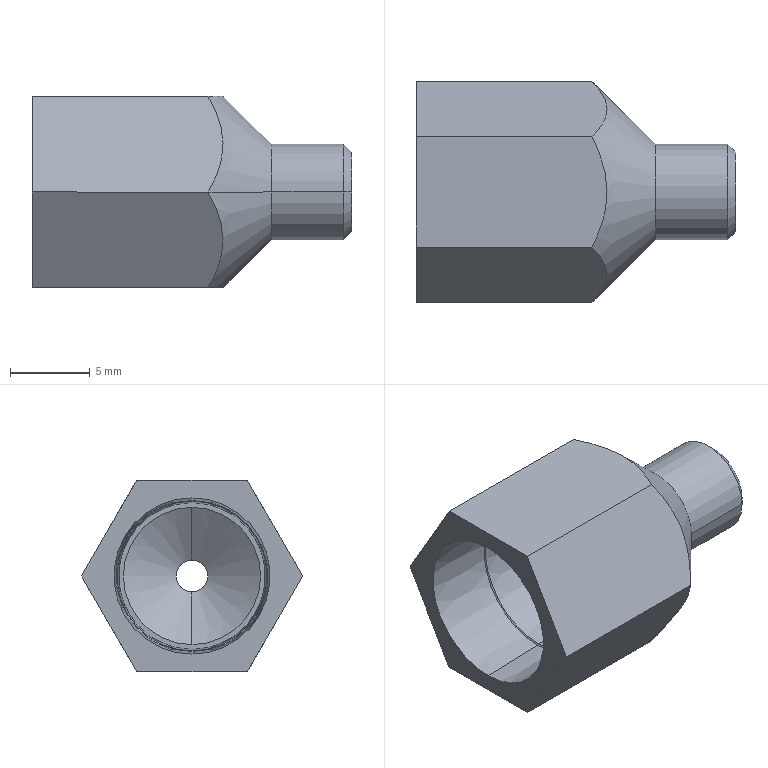Part | STEP file | GN-AD1S-4 | 1 solid | 29 faces | box 20 x 13.856 x 12 mm | volume 884.732 mm3 | cone 12 | plane 9 | cylinder 8 | commonest cylinder face diameters 2 x2 6 x2 8.6 x2 9.2 x2
STEP:
#1=CARTESIAN_POINT('',(4.4,7.61,10.758));
#2=VERTEX_POINT('',#1);
#3=CARTESIAN_POINT('',(4.4,7.61,1.242));
#4=VERTEX_POINT('',#3);
#5=CARTESIAN_POINT('',(4.4,7.61,6.));
#6=DIRECTION('',(1.,0.,0.));
#7=DIRECTION('',(0.,0.,-1.));
#8=AXIS2_PLACEMENT_3D('',#5,#6,#7);
#9=CIRCLE('',#8,4.758);
#10=EDGE_CURVE('',#2,#4,#9,.T.);
#11=ORIENTED_EDGE('',*,*,#10,.T.);
#12=CARTESIAN_POINT('',(0.,7.61,1.105));
#13=VERTEX_POINT('',#12);
#14=CARTESIAN_POINT('',(4.4,7.61,1.242));
#15=DIRECTION('',(-0.9995,0.,-0.0312));
#16=VECTOR('',#15,1000.);
#17=LINE('',#14,#16);
#18=EDGE_CURVE('',#4,#13,#17,.T.);
#19=ORIENTED_EDGE('',*,*,#18,.T.);
#20=CARTESIAN_POINT('',(0.,7.61,10.895));
#21=VERTEX_POINT('',#20);
#22=CARTESIAN_POINT('',(0.,7.61,6.));
#23=DIRECTION('',(-1.,0.,0.));
#24=DIRECTION('',(0.,0.,-1.));
#25=AXIS2_PLACEMENT_3D('',#22,#23,#24);
#26=CIRCLE('',#25,4.895);
#27=EDGE_CURVE('',#13,#21,#26,.T.);
#28=ORIENTED_EDGE('',*,*,#27,.T.);
#29=CARTESIAN_POINT('',(4.4,7.61,10.758));
#30=DIRECTION('',(-0.9995,0.,0.0312));
#31=VECTOR('',#30,1000.);
#32=LINE('',#29,#31);
#33=EDGE_CURVE('',#2,#21,#32,.T.);
#34=ORIENTED_EDGE('',*,*,#33,.F.);
#35=EDGE_LOOP('',(#11,#19,#28,#34));
#36=FACE_OUTER_BOUND('',#35,.T.);
#37=CARTESIAN_POINT('',(4.4,7.61,6.));
#38=DIRECTION('',(-1.,0.,0.));
#39=DIRECTION('',(0.,0.,1.));
#40=AXIS2_PLACEMENT_3D('',#37,#38,#39);
#41=CONICAL_SURFACE('',#40,4.758,0.03121);
#42=ADVANCED_FACE('',(#36),#41,.F.);
#43=CARTESIAN_POINT('',(4.465,7.61,10.693));
#44=VERTEX_POINT('',#43);
#45=CARTESIAN_POINT('',(4.465,7.61,1.307));
#46=VERTEX_POINT('',#45);
#47=CARTESIAN_POINT('',(4.465,7.61,6.));
#48=DIRECTION('',(1.,0.,0.));
#49=DIRECTION('',(0.,0.,-1.));
#50=AXIS2_PLACEMENT_3D('',#47,#48,#49);
#51=CIRCLE('',#50,4.693);
#52=EDGE_CURVE('',#44,#46,#51,.T.);
#53=ORIENTED_EDGE('',*,*,#52,.T.);
#54=CARTESIAN_POINT('',(5.,7.61,1.842));
#55=DIRECTION('',(-0.7071,0.,-0.7071));
#56=VECTOR('',#55,1000.);
#57=LINE('',#54,#56);
#58=EDGE_CURVE('',#46,#4,#57,.T.);
#59=ORIENTED_EDGE('',*,*,#58,.T.);
#60=ORIENTED_EDGE('',*,*,#10,.F.);
#61=CARTESIAN_POINT('',(5.,7.61,10.158));
#62=DIRECTION('',(-0.7071,0.,0.7071));
#63=VECTOR('',#62,1000.);
#64=LINE('',#61,#63);
#65=EDGE_CURVE('',#44,#2,#64,.T.);
#66=ORIENTED_EDGE('',*,*,#65,.F.);
#67=EDGE_LOOP('',(#53,#59,#60,#66));
#68=FACE_OUTER_BOUND('',#67,.T.);
#69=CARTESIAN_POINT('',(5.,7.61,6.));
#70=DIRECTION('',(-1.,0.,0.));
#71=DIRECTION('',(0.,0.,1.));
#72=AXIS2_PLACEMENT_3D('',#69,#70,#71);
#73=CONICAL_SURFACE('',#72,4.158,0.7854);
#74=ADVANCED_FACE('',(#68),#73,.F.);
#75=CARTESIAN_POINT('',(14.983,6.61,6.));
#76=VERTEX_POINT('',#75);
#77=CARTESIAN_POINT('',(14.983,7.61,5.));
#78=VERTEX_POINT('',#77);
#79=CARTESIAN_POINT('',(14.983,7.61,6.));
#80=DIRECTION('',(1.,0.,0.));
#81=DIRECTION('',(0.,0.,1.));
#82=AXIS2_PLACEMENT_3D('',#79,#80,#81);
#83=CIRCLE('',#82,1.);
#84=EDGE_CURVE('',#76,#78,#83,.T.);
#85=ORIENTED_EDGE('',*,*,#84,.F.);
#86=CARTESIAN_POINT('',(20.,6.61,6.));
#87=VERTEX_POINT('',#86);
#88=CARTESIAN_POINT('',(5.,6.61,6.));
#89=DIRECTION('',(1.,0.,0.));
#90=VECTOR('',#89,1000.);
#91=LINE('',#88,#90);
#92=EDGE_CURVE('',#76,#87,#91,.T.);
#93=ORIENTED_EDGE('',*,*,#92,.T.);
#94=CARTESIAN_POINT('',(20.,8.61,6.));
#95=VERTEX_POINT('',#94);
#96=CARTESIAN_POINT('',(20.,7.61,6.));
#97=DIRECTION('',(-1.,0.,0.));
#98=DIRECTION('',(0.,-1.,0.));
#99=AXIS2_PLACEMENT_3D('',#96,#97,#98);
#100=CIRCLE('',#99,1.);
#101=EDGE_CURVE('',#95,#87,#100,.T.);
#102=ORIENTED_EDGE('',*,*,#101,.F.);
#103=CARTESIAN_POINT('',(14.983,8.61,6.));
#104=VERTEX_POINT('',#103);
#105=CARTESIAN_POINT('',(5.,8.61,6.));
#106=DIRECTION('',(1.,0.,0.));
#107=VECTOR('',#106,1000.);
#108=LINE('',#105,#107);
#109=EDGE_CURVE('',#104,#95,#108,.T.);
#110=ORIENTED_EDGE('',*,*,#109,.F.);
#111=CARTESIAN_POINT('',(14.983,7.61,6.));
#112=DIRECTION('',(1.,0.,0.));
#113=DIRECTION('',(0.,0.,1.));
#114=AXIS2_PLACEMENT_3D('',#111,#112,#113);
#115=CIRCLE('',#114,1.);
#116=EDGE_CURVE('',#78,#104,#115,.T.);
#117=ORIENTED_EDGE('',*,*,#116,.F.);
#118=EDGE_LOOP('',(#85,#93,#102,#110,#117));
#119=FACE_OUTER_BOUND('',#118,.T.);
#120=CARTESIAN_POINT('',(5.,7.61,6.));
#121=DIRECTION('',(1.,0.,0.));
#122=DIRECTION('',(0.,1.,0.));
#123=AXIS2_PLACEMENT_3D('',#120,#121,#122);
#124=CYLINDRICAL_SURFACE('',#123,1.);
#125=ADVANCED_FACE('',(#119),#124,.F.);
#126=ORIENTED_EDGE('',*,*,#116,.T.);
#127=CARTESIAN_POINT('',(14.983,7.61,7.));
#128=VERTEX_POINT('',#127);
#129=CARTESIAN_POINT('',(14.983,7.61,6.));
#130=DIRECTION('',(1.,0.,0.));
#131=DIRECTION('',(0.,0.,1.));
#132=AXIS2_PLACEMENT_3D('',#129,#130,#131);
#133=CIRCLE('',#132,1.);
#134=EDGE_CURVE('',#104,#128,#133,.T.);
#135=ORIENTED_EDGE('',*,*,#134,.T.);
#136=CARTESIAN_POINT('',(13.,7.61,10.3));
#137=VERTEX_POINT('',#136);
#138=CARTESIAN_POINT('',(13.,7.61,10.3));
#139=DIRECTION('',(-0.515,0.,0.8572));
#140=VECTOR('',#139,1000.);
#141=LINE('',#138,#140);
#142=EDGE_CURVE('',#128,#137,#141,.T.);
#143=ORIENTED_EDGE('',*,*,#142,.T.);
#144=CARTESIAN_POINT('',(13.,7.61,1.7));
#145=VERTEX_POINT('',#144);
#146=CARTESIAN_POINT('',(13.,7.61,6.));
#147=DIRECTION('',(-1.,0.,0.));
#148=DIRECTION('',(0.,0.,-1.));
#149=AXIS2_PLACEMENT_3D('',#146,#147,#148);
#150=CIRCLE('',#149,4.3);
#151=EDGE_CURVE('',#137,#145,#150,.T.);
#152=ORIENTED_EDGE('',*,*,#151,.T.);
#153=CARTESIAN_POINT('',(13.,7.61,1.7));
#154=DIRECTION('',(-0.515,0.,-0.8572));
#155=VECTOR('',#154,1000.);
#156=LINE('',#153,#155);
#157=EDGE_CURVE('',#78,#145,#156,.T.);
#158=ORIENTED_EDGE('',*,*,#157,.F.);
#159=EDGE_LOOP('',(#126,#135,#143,#152,#158));
#160=FACE_OUTER_BOUND('',#159,.T.);
#161=CARTESIAN_POINT('',(13.,7.61,6.));
#162=DIRECTION('',(-1.,0.,0.));
#163=DIRECTION('',(0.,0.,-1.));
#164=AXIS2_PLACEMENT_3D('',#161,#162,#163);
#165=CONICAL_SURFACE('',#164,4.3,1.03);
#166=ADVANCED_FACE('',(#160),#165,.F.);
#167=ORIENTED_EDGE('',*,*,#151,.F.);
#168=CARTESIAN_POINT('',(10.5,7.61,10.3));
#169=VERTEX_POINT('',#168);
#170=CARTESIAN_POINT('',(-1.,7.61,10.3));
#171=DIRECTION('',(-1.,0.,0.));
#172=VECTOR('',#171,1000.);
#173=LINE('',#170,#172);
#174=EDGE_CURVE('',#137,#169,#173,.T.);
#175=ORIENTED_EDGE('',*,*,#174,.T.);
#176=CARTESIAN_POINT('',(10.5,7.61,1.7));
#177=VERTEX_POINT('',#176);
#178=CARTESIAN_POINT('',(10.5,7.61,6.));
#179=DIRECTION('',(-1.,0.,0.));
#180=DIRECTION('',(0.,0.,-1.));
#181=AXIS2_PLACEMENT_3D('',#178,#179,#180);
#182=CIRCLE('',#181,4.3);
#183=EDGE_CURVE('',#169,#177,#182,.T.);
#184=ORIENTED_EDGE('',*,*,#183,.T.);
#185=CARTESIAN_POINT('',(-1.,7.61,1.7));
#186=DIRECTION('',(-1.,0.,0.));
#187=VECTOR('',#186,1000.);
#188=LINE('',#185,#187);
#189=EDGE_CURVE('',#145,#177,#188,.T.);
#190=ORIENTED_EDGE('',*,*,#189,.F.);
#191=EDGE_LOOP('',(#167,#175,#184,#190));
#192=FACE_OUTER_BOUND('',#191,.T.);
#193=CARTESIAN_POINT('',(-1.,7.61,6.));
#194=DIRECTION('',(-1.,0.,0.));
#195=DIRECTION('',(0.,0.,-1.));
#196=AXIS2_PLACEMENT_3D('',#193,#194,#195);
#197=CYLINDRICAL_SURFACE('',#196,4.3);
#198=ADVANCED_FACE('',(#192),#197,.F.);
#199=CARTESIAN_POINT('',(10.5,7.61,10.6));
#200=VERTEX_POINT('',#199);
#201=CARTESIAN_POINT('',(10.5,7.61,1.4));
#202=VERTEX_POINT('',#201);
#203=CARTESIAN_POINT('',(10.5,7.61,6.));
#204=DIRECTION('',(-1.,0.,0.));
#205=DIRECTION('',(0.,0.,-1.));
#206=AXIS2_PLACEMENT_3D('',#203,#204,#205);
#207=CIRCLE('',#206,4.6);
#208=EDGE_CURVE('',#200,#202,#207,.T.);
#209=ORIENTED_EDGE('',*,*,#208,.F.);
#210=CARTESIAN_POINT('',(7.448,7.61,10.6));
#211=VERTEX_POINT('',#210);
#212=CARTESIAN_POINT('',(-1.,7.61,10.6));
#213=DIRECTION('',(-1.,0.,0.));
#214=VECTOR('',#213,1000.);
#215=LINE('',#212,#214);
#216=EDGE_CURVE('',#200,#211,#215,.T.);
#217=ORIENTED_EDGE('',*,*,#216,.T.);
#218=CARTESIAN_POINT('',(7.448,7.61,1.4));
#219=VERTEX_POINT('',#218);
#220=CARTESIAN_POINT('',(7.448,7.61,6.));
#221=DIRECTION('',(-1.,0.,0.));
#222=DIRECTION('',(0.,0.,-1.));
#223=AXIS2_PLACEMENT_3D('',#220,#221,#222);
#224=CIRCLE('',#223,4.6);
#225=EDGE_CURVE('',#211,#219,#224,.T.);
#226=ORIENTED_EDGE('',*,*,#225,.T.);
#227=CARTESIAN_POINT('',(-1.,7.61,1.4));
#228=DIRECTION('',(-1.,0.,0.));
#229=VECTOR('',#228,1000.);
#230=LINE('',#227,#229);
#231=EDGE_CURVE('',#202,#219,#230,.T.);
#232=ORIENTED_EDGE('',*,*,#231,.F.);
#233=EDGE_LOOP('',(#209,#217,#226,#232));
#234=FACE_OUTER_BOUND('',#233,.T.);
#235=CARTESIAN_POINT('',(-1.,7.61,6.));
#236=DIRECTION('',(-1.,0.,0.));
#237=DIRECTION('',(0.,0.,-1.));
#238=AXIS2_PLACEMENT_3D('',#235,#236,#237);
#239=CYLINDRICAL_SURFACE('',#238,4.6);
#240=ADVANCED_FACE('',(#234),#239,.F.);
#241=ORIENTED_EDGE('',*,*,#225,.F.);
#242=CARTESIAN_POINT('',(-1.,7.61,10.864));
#243=DIRECTION('',(-0.9995,0.,0.03124));
#244=VECTOR('',#243,1000.);
#245=LINE('',#242,#244);
#246=EDGE_CURVE('',#211,#44,#245,.T.);
#247=ORIENTED_EDGE('',*,*,#246,.T.);
#248=CARTESIAN_POINT('',(4.465,7.61,6.));
#249=DIRECTION('',(1.,0.,0.));
#250=DIRECTION('',(0.,0.,-1.));
#251=AXIS2_PLACEMENT_3D('',#248,#249,#250);
#252=CIRCLE('',#251,4.693);
#253=EDGE_CURVE('',#46,#44,#252,.T.);
#254=ORIENTED_EDGE('',*,*,#253,.F.);
#255=CARTESIAN_POINT('',(-1.,7.61,1.136));
#256=DIRECTION('',(-0.9995,0.,-0.03124));
#257=VECTOR('',#256,1000.);
#258=LINE('',#255,#257);
#259=EDGE_CURVE('',#219,#46,#258,.T.);
#260=ORIENTED_EDGE('',*,*,#259,.F.);
#261=EDGE_LOOP('',(#241,#247,#254,#260));
#262=FACE_OUTER_BOUND('',#261,.T.);
#263=CARTESIAN_POINT('',(-1.,7.61,6.));
#264=DIRECTION('',(-1.,0.,0.));
#265=DIRECTION('',(0.,0.,-1.));
#266=AXIS2_PLACEMENT_3D('',#263,#264,#265);
#267=CONICAL_SURFACE('',#266,4.864,0.03124);
#268=ADVANCED_FACE('',(#262),#267,.F.);
#269=CARTESIAN_POINT('',(20.,10.11,6.));
#270=VERTEX_POINT('',#269);
#271=CARTESIAN_POINT('',(20.,5.11,6.));
#272=VERTEX_POINT('',#271);
#273=CARTESIAN_POINT('',(20.,7.61,6.));
#274=DIRECTION('',(1.,0.,0.));
#275=DIRECTION('',(0.,1.,0.));
#276=AXIS2_PLACEMENT_3D('',#273,#274,#275);
#277=CIRCLE('',#276,2.5);
#278=EDGE_CURVE('',#270,#272,#277,.T.);
#279=ORIENTED_EDGE('',*,*,#278,.F.);
#280=CARTESIAN_POINT('',(19.5,10.61,6.));
#281=VERTEX_POINT('',#280);
#282=CARTESIAN_POINT('',(19.5,10.61,6.));
#283=DIRECTION('',(-0.7071,0.7071,0.));
#284=VECTOR('',#283,1000.);
#285=LINE('',#282,#284);
#286=EDGE_CURVE('',#270,#281,#285,.T.);
#287=ORIENTED_EDGE('',*,*,#286,.T.);
#288=CARTESIAN_POINT('',(19.5,4.61,6.));
#289=VERTEX_POINT('',#288);
#290=CARTESIAN_POINT('',(19.5,7.61,6.));
#291=DIRECTION('',(-1.,0.,0.));
#292=DIRECTION('',(0.,1.,0.));
#293=AXIS2_PLACEMENT_3D('',#290,#291,#292);
#294=CIRCLE('',#293,3.);
#295=EDGE_CURVE('',#289,#281,#294,.T.);
#296=ORIENTED_EDGE('',*,*,#295,.F.);
#297=CARTESIAN_POINT('',(19.5,4.61,6.));
#298=DIRECTION('',(-0.7071,-0.7071,0.));
#299=VECTOR('',#298,1000.);
#300=LINE('',#297,#299);
#301=EDGE_CURVE('',#272,#289,#300,.T.);
#302=ORIENTED_EDGE('',*,*,#301,.F.);
#303=EDGE_LOOP('',(#279,#287,#296,#302));
#304=FACE_OUTER_BOUND('',#303,.T.);
#305=CARTESIAN_POINT('',(19.5,7.61,6.));
#306=DIRECTION('',(-1.,0.,0.));
#307=DIRECTION('',(0.,-1.,0.));
#308=AXIS2_PLACEMENT_3D('',#305,#306,#307);
#309=CONICAL_SURFACE('',#308,3.,0.7854);
#310=ADVANCED_FACE('',(#304),#309,.T.);
#311=CARTESIAN_POINT('',(15.,10.61,6.));
#312=VERTEX_POINT('',#311);
#313=CARTESIAN_POINT('',(15.,4.61,6.));
#314=VERTEX_POINT('',#313);
#315=CARTESIAN_POINT('',(15.,7.61,6.));
#316=DIRECTION('',(1.,0.,0.));
#317=DIRECTION('',(0.,1.,0.));
#318=AXIS2_PLACEMENT_3D('',#315,#316,#317);
#319=CIRCLE('',#318,3.);
#320=EDGE_CURVE('',#312,#314,#319,.T.);
#321=ORIENTED_EDGE('',*,*,#320,.T.);
#322=CARTESIAN_POINT('',(15.,4.61,6.));
#323=DIRECTION('',(1.,0.,0.));
#324=VECTOR('',#323,1000.);
#325=LINE('',#322,#324);
#326=EDGE_CURVE('',#314,#289,#325,.T.);
#327=ORIENTED_EDGE('',*,*,#326,.T.);
#328=ORIENTED_EDGE('',*,*,#295,.T.);
#329=CARTESIAN_POINT('',(15.,10.61,6.));
#330=DIRECTION('',(1.,0.,0.));
#331=VECTOR('',#330,1000.);
#332=LINE('',#329,#331);
#333=EDGE_CURVE('',#312,#281,#332,.T.);
#334=ORIENTED_EDGE('',*,*,#333,.F.);
#335=EDGE_LOOP('',(#321,#327,#328,#334));
#336=FACE_OUTER_BOUND('',#335,.T.);
#337=CARTESIAN_POINT('',(15.,7.61,6.));
#338=DIRECTION('',(1.,0.,0.));
#339=DIRECTION('',(0.,1.,0.));
#340=AXIS2_PLACEMENT_3D('',#337,#338,#339);
#341=CYLINDRICAL_SURFACE('',#340,3.);
#342=ADVANCED_FACE('',(#336),#341,.T.);
#343=ORIENTED_EDGE('',*,*,#320,.F.);
#344=CARTESIAN_POINT('',(11.,14.538,6.));
#345=VERTEX_POINT('',#344);
#346=CARTESIAN_POINT('',(15.,10.61,6.));
#347=DIRECTION('',(-0.7135,0.7007,0.));
#348=VECTOR('',#347,1000.);
#349=LINE('',#346,#348);
#350=EDGE_CURVE('',#312,#345,#349,.T.);
#351=ORIENTED_EDGE('',*,*,#350,.T.);
#352=CARTESIAN_POINT('',(11.,11.074,12.));
#353=VERTEX_POINT('',#352);
#354=CARTESIAN_POINT('',(11.,11.074,12.));
#355=CARTESIAN_POINT('',(11.275,11.344,11.532));
#356=CARTESIAN_POINT('',(11.509,11.621,11.053));
#357=CARTESIAN_POINT('',(11.761,12.051,10.308));
#358=CARTESIAN_POINT('',(11.828,12.197,10.056));
#359=CARTESIAN_POINT('',(11.92,12.495,9.539));
#360=CARTESIAN_POINT('',(11.945,12.649,9.273));
#361=CARTESIAN_POINT('',(11.946,13.103,8.486));
#362=CARTESIAN_POINT('',(11.853,13.401,7.97));
#363=CARTESIAN_POINT('',(11.514,13.987,6.954));
#364=CARTESIAN_POINT('',(11.277,14.267,6.47));
#365=CARTESIAN_POINT('',(11.,14.538,6.));
#366=B_SPLINE_CURVE_WITH_KNOTS('',3,(#354,#355,#356,#357,#358,#359,#360,#361,#362,#363,#364,#365),.UNSPECIFIED.,.F.,.F.,(4,2,2,2,2,4),(0.000000255,0.001792,0.002688,0.003584,0.005376,0.007168),.UNSPECIFIED.);
#367=EDGE_CURVE('',#353,#345,#366,.T.);
#368=ORIENTED_EDGE('',*,*,#367,.F.);
#369=CARTESIAN_POINT('',(11.,4.146,12.));
#370=VERTEX_POINT('',#369);
#371=CARTESIAN_POINT('',(11.,4.146,12.));
#372=CARTESIAN_POINT('',(11.274,4.685,12.));
#373=CARTESIAN_POINT('',(11.51,5.239,12.));
#374=CARTESIAN_POINT('',(11.765,6.115,12.));
#375=CARTESIAN_POINT('',(11.832,6.411,12.));
#376=CARTESIAN_POINT('',(11.922,7.006,12.));
#377=CARTESIAN_POINT('',(11.945,7.306,12.));
#378=CARTESIAN_POINT('',(11.945,7.91,12.));
#379=CARTESIAN_POINT('',(11.922,8.216,12.));
#380=CARTESIAN_POINT('',(11.831,8.814,12.));
#381=CARTESIAN_POINT('',(11.764,9.107,12.));
#382=CARTESIAN_POINT('',(11.596,9.687,12.));
#383=CARTESIAN_POINT('',(11.493,9.974,12.));
#384=CARTESIAN_POINT('',(11.263,10.534,12.));
#385=CARTESIAN_POINT('',(11.136,10.807,12.));
#386=CARTESIAN_POINT('',(11.,11.074,12.));
#387=B_SPLINE_CURVE_WITH_KNOTS('',3,(#371,#372,#373,#374,#375,#376,#377,#378,#379,#380,#381,#382,#383,#384,#385,#386),.UNSPECIFIED.,.F.,.F.,(4,2,2,2,2,2,2,4),(0.01194,0.01376,0.01466,0.01557,0.01647,0.01738,0.01829,0.01919),.UNSPECIFIED.);
#388=EDGE_CURVE('',#370,#353,#387,.T.);
#389=ORIENTED_EDGE('',*,*,#388,.F.);
#390=CARTESIAN_POINT('',(11.,0.6823,6.));
#391=VERTEX_POINT('',#390);
#392=CARTESIAN_POINT('',(11.,0.6823,6.));
#393=CARTESIAN_POINT('',(11.275,0.9523,6.468));
#394=CARTESIAN_POINT('',(11.509,1.229,6.946));
#395=CARTESIAN_POINT('',(11.761,1.659,7.691));
#396=CARTESIAN_POINT('',(11.828,1.805,7.944));
#397=CARTESIAN_POINT('',(11.92,2.103,8.461));
#398=CARTESIAN_POINT('',(11.945,2.257,8.727));
#399=CARTESIAN_POINT('',(11.946,2.711,9.513));
#400=CARTESIAN_POINT('',(11.853,3.009,10.03));
#401=CARTESIAN_POINT('',(11.514,3.595,11.045));
#402=CARTESIAN_POINT('',(11.277,3.875,11.529));
#403=CARTESIAN_POINT('',(11.,4.146,12.));
#404=B_SPLINE_CURVE_WITH_KNOTS('',3,(#392,#393,#394,#395,#396,#397,#398,#399,#400,#401,#402,#403),.UNSPECIFIED.,.F.,.F.,(4,2,2,2,2,4),(0.000000255,0.001792,0.002688,0.003584,0.005376,0.007168),.UNSPECIFIED.);
#405=EDGE_CURVE('',#391,#370,#404,.T.);
#406=ORIENTED_EDGE('',*,*,#405,.F.);
#407=CARTESIAN_POINT('',(15.,4.61,6.));
#408=DIRECTION('',(-0.7135,-0.7007,0.));
#409=VECTOR('',#408,1000.);
#410=LINE('',#407,#409);
#411=EDGE_CURVE('',#314,#391,#410,.T.);
#412=ORIENTED_EDGE('',*,*,#411,.F.);
#413=EDGE_LOOP('',(#343,#351,#368,#389,#406,#412));
#414=FACE_OUTER_BOUND('',#413,.T.);
#415=CARTESIAN_POINT('',(15.,7.61,6.));
#416=DIRECTION('',(-1.,0.,0.));
#417=DIRECTION('',(0.,-1.,0.));
#418=AXIS2_PLACEMENT_3D('',#415,#416,#417);
#419=CONICAL_SURFACE('',#418,3.,0.7763);
#420=ADVANCED_FACE('',(#414),#419,.T.);
#421=CARTESIAN_POINT('',(0.,11.074,0.));
#422=VERTEX_POINT('',#421);
#423=CARTESIAN_POINT('',(0.,14.538,6.));
#424=VERTEX_POINT('',#423);
#425=CARTESIAN_POINT('',(0.,11.074,0.));
#426=DIRECTION('',(0.,0.5,0.866));
#427=VECTOR('',#426,1000.);
#428=LINE('',#425,#427);
#429=EDGE_CURVE('',#422,#424,#428,.T.);
#430=ORIENTED_EDGE('',*,*,#429,.T.);
#431=CARTESIAN_POINT('',(11.,14.538,6.));
#432=DIRECTION('',(-1.,0.,0.));
#433=VECTOR('',#432,1000.);
#434=LINE('',#431,#433);
#435=EDGE_CURVE('',#345,#424,#434,.T.);
#436=ORIENTED_EDGE('',*,*,#435,.F.);
#437=CARTESIAN_POINT('',(11.,11.074,0.));
#438=VERTEX_POINT('',#437);
#439=CARTESIAN_POINT('',(11.,14.538,6.));
#440=CARTESIAN_POINT('',(11.275,14.268,5.532));
#441=CARTESIAN_POINT('',(11.509,13.992,5.053));
#442=CARTESIAN_POINT('',(11.761,13.562,4.309));
#443=CARTESIAN_POINT('',(11.828,13.416,4.056));
#444=CARTESIAN_POINT('',(11.92,13.117,3.539));
#445=CARTESIAN_POINT('',(11.945,12.964,3.273));
#446=CARTESIAN_POINT('',(11.946,12.51,2.487));
#447=CARTESIAN_POINT('',(11.853,12.211,1.97));
#448=CARTESIAN_POINT('',(11.514,11.625,0.9545));
#449=CARTESIAN_POINT('',(11.277,11.346,0.4704));
#450=CARTESIAN_POINT('',(11.,11.074,0.));
#451=B_SPLINE_CURVE_WITH_KNOTS('',3,(#439,#440,#441,#442,#443,#444,#445,#446,#447,#448,#449,#450),.UNSPECIFIED.,.F.,.F.,(4,2,2,2,2,4),(0.000000255,0.001792,0.002688,0.003584,0.005376,0.007168),.UNSPECIFIED.);
#452=EDGE_CURVE('',#345,#438,#451,.T.);
#453=ORIENTED_EDGE('',*,*,#452,.T.);
#454=CARTESIAN_POINT('',(11.,11.074,0.));
#455=DIRECTION('',(-1.,0.,0.));
#456=VECTOR('',#455,1000.);
#457=LINE('',#454,#456);
#458=EDGE_CURVE('',#438,#422,#457,.T.);
#459=ORIENTED_EDGE('',*,*,#458,.T.);
#460=EDGE_LOOP('',(#430,#436,#453,#459));
#461=FACE_OUTER_BOUND('',#460,.T.);
#462=CARTESIAN_POINT('',(11.,11.074,0.));
#463=DIRECTION('',(0.,-0.866,0.5));
#464=DIRECTION('',(0.,-0.5,-0.866));
#465=AXIS2_PLACEMENT_3D('',#462,#463,#464);
#466=PLANE('',#465);
#467=ADVANCED_FACE('',(#461),#466,.F.);
#468=CARTESIAN_POINT('',(0.,11.074,12.));
#469=VERTEX_POINT('',#468);
#470=CARTESIAN_POINT('',(0.,14.538,6.));
#471=DIRECTION('',(0.,-0.5,0.866));
#472=VECTOR('',#471,1000.);
#473=LINE('',#470,#472);
#474=EDGE_CURVE('',#424,#469,#473,.T.);
#475=ORIENTED_EDGE('',*,*,#474,.T.);
#476=CARTESIAN_POINT('',(11.,11.074,12.));
#477=DIRECTION('',(-1.,0.,0.));
#478=VECTOR('',#477,1000.);
#479=LINE('',#476,#478);
#480=EDGE_CURVE('',#353,#469,#479,.T.);
#481=ORIENTED_EDGE('',*,*,#480,.F.);
#482=ORIENTED_EDGE('',*,*,#367,.T.);
#483=ORIENTED_EDGE('',*,*,#435,.T.);
#484=EDGE_LOOP('',(#475,#481,#482,#483));
#485=FACE_OUTER_BOUND('',#484,.T.);
#486=CARTESIAN_POINT('',(11.,14.538,6.));
#487=DIRECTION('',(0.,-0.866,-0.5));
#488=DIRECTION('',(0.,0.5,-0.866));
#489=AXIS2_PLACEMENT_3D('',#486,#487,#488);
#490=PLANE('',#489);
#491=ADVANCED_FACE('',(#485),#490,.F.);
#492=CARTESIAN_POINT('',(0.,4.146,12.));
#493=VERTEX_POINT('',#492);
#494=CARTESIAN_POINT('',(0.,11.074,12.));
#495=DIRECTION('',(0.,-1.,0.));
#496=VECTOR('',#495,1000.);
#497=LINE('',#494,#496);
#498=EDGE_CURVE('',#469,#493,#497,.T.);
#499=ORIENTED_EDGE('',*,*,#498,.T.);
#500=CARTESIAN_POINT('',(11.,4.146,12.));
#501=DIRECTION('',(-1.,0.,0.));
#502=VECTOR('',#501,1000.);
#503=LINE('',#500,#502);
#504=EDGE_CURVE('',#370,#493,#503,.T.);
#505=ORIENTED_EDGE('',*,*,#504,.F.);
#506=ORIENTED_EDGE('',*,*,#388,.T.);
#507=ORIENTED_EDGE('',*,*,#480,.T.);
#508=EDGE_LOOP('',(#499,#505,#506,#507));
#509=FACE_OUTER_BOUND('',#508,.T.);
#510=CARTESIAN_POINT('',(11.,11.074,12.));
#511=DIRECTION('',(0.,0.,-1.));
#512=DIRECTION('',(0.,1.,0.));
#513=AXIS2_PLACEMENT_3D('',#510,#511,#512);
#514=PLANE('',#513);
#515=ADVANCED_FACE('',(#509),#514,.F.);
#516=CARTESIAN_POINT('',(0.,0.6823,6.));
#517=VERTEX_POINT('',#516);
#518=CARTESIAN_POINT('',(0.,4.146,12.));
#519=DIRECTION('',(0.,-0.5,-0.866));
#520=VECTOR('',#519,1000.);
#521=LINE('',#518,#520);
#522=EDGE_CURVE('',#493,#517,#521,.T.);
#523=ORIENTED_EDGE('',*,*,#522,.T.);
#524=CARTESIAN_POINT('',(11.,0.6823,6.));
#525=DIRECTION('',(-1.,0.,0.));
#526=VECTOR('',#525,1000.);
#527=LINE('',#524,#526);
#528=EDGE_CURVE('',#391,#517,#527,.T.);
#529=ORIENTED_EDGE('',*,*,#528,.F.);
#530=ORIENTED_EDGE('',*,*,#405,.T.);
#531=ORIENTED_EDGE('',*,*,#504,.T.);
#532=EDGE_LOOP('',(#523,#529,#530,#531));
#533=FACE_OUTER_BOUND('',#532,.T.);
#534=CARTESIAN_POINT('',(11.,4.146,12.));
#535=DIRECTION('',(0.,0.866,-0.5));
#536=DIRECTION('',(0.,0.5,0.866));
#537=AXIS2_PLACEMENT_3D('',#534,#535,#536);
#538=PLANE('',#537);
#539=ADVANCED_FACE('',(#533),#538,.F.);
#540=CARTESIAN_POINT('',(0.,4.146,0.));
#541=VERTEX_POINT('',#540);
#542=CARTESIAN_POINT('',(0.,0.6823,6.));
#543=DIRECTION('',(0.,0.5,-0.866));
#544=VECTOR('',#543,1000.);
#545=LINE('',#542,#544);
#546=EDGE_CURVE('',#517,#541,#545,.T.);
#547=ORIENTED_EDGE('',*,*,#546,.T.);
#548=CARTESIAN_POINT('',(11.,4.146,0.));
#549=VERTEX_POINT('',#548);
#550=CARTESIAN_POINT('',(11.,4.146,0.));
#551=DIRECTION('',(-1.,0.,0.));
#552=VECTOR('',#551,1000.);
#553=LINE('',#550,#552);
#554=EDGE_CURVE('',#549,#541,#553,.T.);
#555=ORIENTED_EDGE('',*,*,#554,.F.);
#556=CARTESIAN_POINT('',(11.,4.146,0.));
#557=CARTESIAN_POINT('',(11.275,3.876,0.4677));
#558=CARTESIAN_POINT('',(11.509,3.6,0.9464));
#559=CARTESIAN_POINT('',(11.761,3.17,1.691));
#560=CARTESIAN_POINT('',(11.828,3.024,1.944));
#561=CARTESIAN_POINT('',(11.92,2.725,2.461));
#562=CARTESIAN_POINT('',(11.945,2.572,2.727));
#563=CARTESIAN_POINT('',(11.946,2.118,3.513));
#564=CARTESIAN_POINT('',(11.853,1.819,4.03));
#565=CARTESIAN_POINT('',(11.514,1.233,5.045));
#566=CARTESIAN_POINT('',(11.277,0.9539,5.529));
#567=CARTESIAN_POINT('',(11.,0.6823,6.));
#568=B_SPLINE_CURVE_WITH_KNOTS('',3,(#556,#557,#558,#559,#560,#561,#562,#563,#564,#565,#566,#567),.UNSPECIFIED.,.F.,.F.,(4,2,2,2,2,4),(0.000000255,0.001792,0.002688,0.003584,0.005376,0.007168),.UNSPECIFIED.);
#569=EDGE_CURVE('',#549,#391,#568,.T.);
#570=ORIENTED_EDGE('',*,*,#569,.T.);
#571=ORIENTED_EDGE('',*,*,#528,.T.);
#572=EDGE_LOOP('',(#547,#555,#570,#571));
#573=FACE_OUTER_BOUND('',#572,.T.);
#574=CARTESIAN_POINT('',(11.,0.6823,6.));
#575=DIRECTION('',(0.,0.866,0.5));
#576=DIRECTION('',(0.,-0.5,0.866));
#577=AXIS2_PLACEMENT_3D('',#574,#575,#576);
#578=PLANE('',#577);
#579=ADVANCED_FACE('',(#573),#578,.F.);
#580=CARTESIAN_POINT('',(0.,4.146,0.));
#581=DIRECTION('',(0.,1.,0.));
#582=VECTOR('',#581,1000.);
#583=LINE('',#580,#582);
#584=EDGE_CURVE('',#541,#422,#583,.T.);
#585=ORIENTED_EDGE('',*,*,#584,.T.);
#586=ORIENTED_EDGE('',*,*,#458,.F.);
#587=CARTESIAN_POINT('',(11.,11.074,0.));
#588=CARTESIAN_POINT('',(11.274,10.536,0.));
#589=CARTESIAN_POINT('',(11.51,9.981,0.));
#590=CARTESIAN_POINT('',(11.765,9.106,0.));
#591=CARTESIAN_POINT('',(11.832,8.809,0.));
#592=CARTESIAN_POINT('',(11.922,8.215,0.));
#593=CARTESIAN_POINT('',(11.945,7.915,0.));
#594=CARTESIAN_POINT('',(11.945,7.311,0.));
#595=CARTESIAN_POINT('',(11.922,7.005,0.));
#596=CARTESIAN_POINT('',(11.831,6.407,0.));
#597=CARTESIAN_POINT('',(11.764,6.113,0.));
#598=CARTESIAN_POINT('',(11.596,5.534,0.));
#599=CARTESIAN_POINT('',(11.493,5.247,0.));
#600=CARTESIAN_POINT('',(11.263,4.686,0.));
#601=CARTESIAN_POINT('',(11.136,4.414,0.));
#602=CARTESIAN_POINT('',(11.,4.146,0.));
#603=B_SPLINE_CURVE_WITH_KNOTS('',3,(#587,#588,#589,#590,#591,#592,#593,#594,#595,#596,#597,#598,#599,#600,#601,#602),.UNSPECIFIED.,.F.,.F.,(4,2,2,2,2,2,2,4),(0.01194,0.01376,0.01466,0.01557,0.01647,0.01738,0.01829,0.01919),.UNSPECIFIED.);
#604=EDGE_CURVE('',#438,#549,#603,.T.);
#605=ORIENTED_EDGE('',*,*,#604,.T.);
#606=ORIENTED_EDGE('',*,*,#554,.T.);
#607=EDGE_LOOP('',(#585,#586,#605,#606));
#608=FACE_OUTER_BOUND('',#607,.T.);
#609=CARTESIAN_POINT('',(11.,4.146,0.));
#610=DIRECTION('',(0.,0.,1.));
#611=DIRECTION('',(0.,-1.,0.));
#612=AXIS2_PLACEMENT_3D('',#609,#610,#611);
#613=PLANE('',#612);
#614=ADVANCED_FACE('',(#608),#613,.F.);
#615=CARTESIAN_POINT('',(0.,7.61,6.));
#616=DIRECTION('',(-1.,0.,0.));
#617=DIRECTION('',(0.,0.,-1.));
#618=AXIS2_PLACEMENT_3D('',#615,#616,#617);
#619=CIRCLE('',#618,4.895);
#620=EDGE_CURVE('',#21,#13,#619,.T.);
#621=ORIENTED_EDGE('',*,*,#620,.F.);
#622=ORIENTED_EDGE('',*,*,#27,.F.);
#623=EDGE_LOOP('',(#621,#622));
#624=FACE_BOUND('',#623,.T.);
#625=ORIENTED_EDGE('',*,*,#429,.F.);
#626=ORIENTED_EDGE('',*,*,#584,.F.);
#627=ORIENTED_EDGE('',*,*,#546,.F.);
#628=ORIENTED_EDGE('',*,*,#522,.F.);
#629=ORIENTED_EDGE('',*,*,#498,.F.);
#630=ORIENTED_EDGE('',*,*,#474,.F.);
#631=EDGE_LOOP('',(#625,#626,#627,#628,#629,#630));
#632=FACE_OUTER_BOUND('',#631,.T.);
#633=CARTESIAN_POINT('',(0.,7.61,6.));
#634=DIRECTION('',(1.,0.,0.));
#635=DIRECTION('',(0.,1.,0.));
#636=AXIS2_PLACEMENT_3D('',#633,#634,#635);
#637=PLANE('',#636);
#638=ADVANCED_FACE('',(#624,#632),#637,.F.);
#639=ORIENTED_EDGE('',*,*,#350,.F.);
#640=CARTESIAN_POINT('',(15.,7.61,6.));
#641=DIRECTION('',(1.,0.,0.));
#642=DIRECTION('',(0.,1.,0.));
#643=AXIS2_PLACEMENT_3D('',#640,#641,#642);
#644=CIRCLE('',#643,3.);
#645=EDGE_CURVE('',#314,#312,#644,.T.);
#646=ORIENTED_EDGE('',*,*,#645,.F.);
#647=ORIENTED_EDGE('',*,*,#411,.T.);
#648=ORIENTED_EDGE('',*,*,#569,.F.);
#649=ORIENTED_EDGE('',*,*,#604,.F.);
#650=ORIENTED_EDGE('',*,*,#452,.F.);
#651=EDGE_LOOP('',(#639,#646,#647,#648,#649,#650));
#652=FACE_OUTER_BOUND('',#651,.T.);
#653=CARTESIAN_POINT('',(15.,7.61,6.));
#654=DIRECTION('',(-1.,0.,0.));
#655=DIRECTION('',(0.,-1.,0.));
#656=AXIS2_PLACEMENT_3D('',#653,#654,#655);
#657=CONICAL_SURFACE('',#656,3.,0.7763);
#658=ADVANCED_FACE('',(#652),#657,.T.);
#659=ORIENTED_EDGE('',*,*,#101,.T.);
#660=CARTESIAN_POINT('',(20.,7.61,6.));
#661=DIRECTION('',(-1.,0.,0.));
#662=DIRECTION('',(0.,-1.,0.));
#663=AXIS2_PLACEMENT_3D('',#660,#661,#662);
#664=CIRCLE('',#663,1.);
#665=EDGE_CURVE('',#87,#95,#664,.T.);
#666=ORIENTED_EDGE('',*,*,#665,.T.);
#667=EDGE_LOOP('',(#659,#666));
#668=FACE_BOUND('',#667,.T.);
#669=CARTESIAN_POINT('',(20.,7.61,6.));
#670=DIRECTION('',(1.,0.,0.));
#671=DIRECTION('',(0.,1.,0.));
#672=AXIS2_PLACEMENT_3D('',#669,#670,#671);
#673=CIRCLE('',#672,2.5);
#674=EDGE_CURVE('',#272,#270,#673,.T.);
#675=ORIENTED_EDGE('',*,*,#674,.T.);
#676=ORIENTED_EDGE('',*,*,#278,.T.);
#677=EDGE_LOOP('',(#675,#676));
#678=FACE_OUTER_BOUND('',#677,.T.);
#679=CARTESIAN_POINT('',(20.,7.61,6.));
#680=DIRECTION('',(1.,0.,0.));
#681=DIRECTION('',(0.,1.,0.));
#682=AXIS2_PLACEMENT_3D('',#679,#680,#681);
#683=PLANE('',#682);
#684=ADVANCED_FACE('',(#668,#678),#683,.T.);
#685=ORIENTED_EDGE('',*,*,#326,.F.);
#686=ORIENTED_EDGE('',*,*,#645,.T.);
#687=ORIENTED_EDGE('',*,*,#333,.T.);
#688=CARTESIAN_POINT('',(19.5,7.61,6.));
#689=DIRECTION('',(-1.,0.,0.));
#690=DIRECTION('',(0.,1.,0.));
#691=AXIS2_PLACEMENT_3D('',#688,#689,#690);
#692=CIRCLE('',#691,3.);
#693=EDGE_CURVE('',#281,#289,#692,.T.);
#694=ORIENTED_EDGE('',*,*,#693,.T.);
#695=EDGE_LOOP('',(#685,#686,#687,#694));
#696=FACE_OUTER_BOUND('',#695,.T.);
#697=CARTESIAN_POINT('',(15.,7.61,6.));
#698=DIRECTION('',(1.,0.,0.));
#699=DIRECTION('',(0.,1.,0.));
#700=AXIS2_PLACEMENT_3D('',#697,#698,#699);
#701=CYLINDRICAL_SURFACE('',#700,3.);
#702=ADVANCED_FACE('',(#696),#701,.T.);
#703=ORIENTED_EDGE('',*,*,#286,.F.);
#704=ORIENTED_EDGE('',*,*,#674,.F.);
#705=ORIENTED_EDGE('',*,*,#301,.T.);
#706=ORIENTED_EDGE('',*,*,#693,.F.);
#707=EDGE_LOOP('',(#703,#704,#705,#706));
#708=FACE_OUTER_BOUND('',#707,.T.);
#709=CARTESIAN_POINT('',(19.5,7.61,6.));
#710=DIRECTION('',(-1.,0.,0.));
#711=DIRECTION('',(0.,-1.,0.));
#712=AXIS2_PLACEMENT_3D('',#709,#710,#711);
#713=CONICAL_SURFACE('',#712,3.,0.7854);
#714=ADVANCED_FACE('',(#708),#713,.T.);
#715=ORIENTED_EDGE('',*,*,#246,.F.);
#716=CARTESIAN_POINT('',(7.448,7.61,6.));
#717=DIRECTION('',(-1.,0.,0.));
#718=DIRECTION('',(0.,0.,-1.));
#719=AXIS2_PLACEMENT_3D('',#716,#717,#718);
#720=CIRCLE('',#719,4.6);
#721=EDGE_CURVE('',#219,#211,#720,.T.);
#722=ORIENTED_EDGE('',*,*,#721,.F.);
#723=ORIENTED_EDGE('',*,*,#259,.T.);
#724=ORIENTED_EDGE('',*,*,#52,.F.);
#725=EDGE_LOOP('',(#715,#722,#723,#724));
#726=FACE_OUTER_BOUND('',#725,.T.);
#727=CARTESIAN_POINT('',(-1.,7.61,6.));
#728=DIRECTION('',(-1.,0.,0.));
#729=DIRECTION('',(0.,0.,-1.));
#730=AXIS2_PLACEMENT_3D('',#727,#728,#729);
#731=CONICAL_SURFACE('',#730,4.864,0.03124);
#732=ADVANCED_FACE('',(#726),#731,.F.);
#733=ORIENTED_EDGE('',*,*,#216,.F.);
#734=CARTESIAN_POINT('',(10.5,7.61,6.));
#735=DIRECTION('',(-1.,0.,0.));
#736=DIRECTION('',(0.,0.,-1.));
#737=AXIS2_PLACEMENT_3D('',#734,#735,#736);
#738=CIRCLE('',#737,4.6);
#739=EDGE_CURVE('',#202,#200,#738,.T.);
#740=ORIENTED_EDGE('',*,*,#739,.F.);
#741=ORIENTED_EDGE('',*,*,#231,.T.);
#742=ORIENTED_EDGE('',*,*,#721,.T.);
#743=EDGE_LOOP('',(#733,#740,#741,#742));
#744=FACE_OUTER_BOUND('',#743,.T.);
#745=CARTESIAN_POINT('',(-1.,7.61,6.));
#746=DIRECTION('',(-1.,0.,0.));
#747=DIRECTION('',(0.,0.,-1.));
#748=AXIS2_PLACEMENT_3D('',#745,#746,#747);
#749=CYLINDRICAL_SURFACE('',#748,4.6);
#750=ADVANCED_FACE('',(#744),#749,.F.);
#751=CARTESIAN_POINT('',(10.5,7.61,6.));
#752=DIRECTION('',(-1.,0.,0.));
#753=DIRECTION('',(0.,0.,-1.));
#754=AXIS2_PLACEMENT_3D('',#751,#752,#753);
#755=CIRCLE('',#754,4.3);
#756=EDGE_CURVE('',#177,#169,#755,.T.);
#757=ORIENTED_EDGE('',*,*,#756,.F.);
#758=ORIENTED_EDGE('',*,*,#183,.F.);
#759=EDGE_LOOP('',(#757,#758));
#760=FACE_BOUND('',#759,.T.);
#761=ORIENTED_EDGE('',*,*,#739,.T.);
#762=ORIENTED_EDGE('',*,*,#208,.T.);
#763=EDGE_LOOP('',(#761,#762));
#764=FACE_OUTER_BOUND('',#763,.T.);
#765=CARTESIAN_POINT('',(10.5,7.61,10.6));
#766=DIRECTION('',(1.,0.,0.));
#767=DIRECTION('',(0.,0.,1.));
#768=AXIS2_PLACEMENT_3D('',#765,#766,#767);
#769=PLANE('',#768);
#770=ADVANCED_FACE('',(#760,#764),#769,.F.);
#771=ORIENTED_EDGE('',*,*,#174,.F.);
#772=CARTESIAN_POINT('',(13.,7.61,6.));
#773=DIRECTION('',(-1.,0.,0.));
#774=DIRECTION('',(0.,0.,-1.));
#775=AXIS2_PLACEMENT_3D('',#772,#773,#774);
#776=CIRCLE('',#775,4.3);
#777=EDGE_CURVE('',#145,#137,#776,.T.);
#778=ORIENTED_EDGE('',*,*,#777,.F.);
#779=ORIENTED_EDGE('',*,*,#189,.T.);
#780=ORIENTED_EDGE('',*,*,#756,.T.);
#781=EDGE_LOOP('',(#771,#778,#779,#780));
#782=FACE_OUTER_BOUND('',#781,.T.);
#783=CARTESIAN_POINT('',(-1.,7.61,6.));
#784=DIRECTION('',(-1.,0.,0.));
#785=DIRECTION('',(0.,0.,-1.));
#786=AXIS2_PLACEMENT_3D('',#783,#784,#785);
#787=CYLINDRICAL_SURFACE('',#786,4.3);
#788=ADVANCED_FACE('',(#782),#787,.F.);
#789=ORIENTED_EDGE('',*,*,#142,.F.);
#790=CARTESIAN_POINT('',(14.983,7.61,6.));
#791=DIRECTION('',(1.,0.,0.));
#792=DIRECTION('',(0.,0.,1.));
#793=AXIS2_PLACEMENT_3D('',#790,#791,#792);
#794=CIRCLE('',#793,1.);
#795=EDGE_CURVE('',#128,#76,#794,.T.);
#796=ORIENTED_EDGE('',*,*,#795,.T.);
#797=ORIENTED_EDGE('',*,*,#84,.T.);
#798=ORIENTED_EDGE('',*,*,#157,.T.);
#799=ORIENTED_EDGE('',*,*,#777,.T.);
#800=EDGE_LOOP('',(#789,#796,#797,#798,#799));
#801=FACE_OUTER_BOUND('',#800,.T.);
#802=CARTESIAN_POINT('',(13.,7.61,6.));
#803=DIRECTION('',(-1.,0.,0.));
#804=DIRECTION('',(0.,0.,-1.));
#805=AXIS2_PLACEMENT_3D('',#802,#803,#804);
#806=CONICAL_SURFACE('',#805,4.3,1.03);
#807=ADVANCED_FACE('',(#801),#806,.F.);
#808=ORIENTED_EDGE('',*,*,#92,.F.);
#809=ORIENTED_EDGE('',*,*,#795,.F.);
#810=ORIENTED_EDGE('',*,*,#134,.F.);
#811=ORIENTED_EDGE('',*,*,#109,.T.);
#812=ORIENTED_EDGE('',*,*,#665,.F.);
#813=EDGE_LOOP('',(#808,#809,#810,#811,#812));
#814=FACE_OUTER_BOUND('',#813,.T.);
#815=CARTESIAN_POINT('',(5.,7.61,6.));
#816=DIRECTION('',(1.,0.,0.));
#817=DIRECTION('',(0.,1.,0.));
#818=AXIS2_PLACEMENT_3D('',#815,#816,#817);
#819=CYLINDRICAL_SURFACE('',#818,1.);
#820=ADVANCED_FACE('',(#814),#819,.F.);
#821=ORIENTED_EDGE('',*,*,#58,.F.);
#822=ORIENTED_EDGE('',*,*,#253,.T.);
#823=ORIENTED_EDGE('',*,*,#65,.T.);
#824=CARTESIAN_POINT('',(4.4,7.61,6.));
#825=DIRECTION('',(1.,0.,0.));
#826=DIRECTION('',(0.,0.,-1.));
#827=AXIS2_PLACEMENT_3D('',#824,#825,#826);
#828=CIRCLE('',#827,4.758);
#829=EDGE_CURVE('',#4,#2,#828,.T.);
#830=ORIENTED_EDGE('',*,*,#829,.F.);
#831=EDGE_LOOP('',(#821,#822,#823,#830));
#832=FACE_OUTER_BOUND('',#831,.T.);
#833=CARTESIAN_POINT('',(5.,7.61,6.));
#834=DIRECTION('',(-1.,0.,0.));
#835=DIRECTION('',(0.,0.,1.));
#836=AXIS2_PLACEMENT_3D('',#833,#834,#835);
#837=CONICAL_SURFACE('',#836,4.158,0.7854);
#838=ADVANCED_FACE('',(#832),#837,.F.);
#839=ORIENTED_EDGE('',*,*,#18,.F.);
#840=ORIENTED_EDGE('',*,*,#829,.T.);
#841=ORIENTED_EDGE('',*,*,#33,.T.);
#842=ORIENTED_EDGE('',*,*,#620,.T.);
#843=EDGE_LOOP('',(#839,#840,#841,#842));
#844=FACE_OUTER_BOUND('',#843,.T.);
#845=CARTESIAN_POINT('',(4.4,7.61,6.));
#846=DIRECTION('',(-1.,0.,0.));
#847=DIRECTION('',(0.,0.,1.));
#848=AXIS2_PLACEMENT_3D('',#845,#846,#847);
#849=CONICAL_SURFACE('',#848,4.758,0.03121);
#850=ADVANCED_FACE('',(#844),#849,.F.);
#851=CLOSED_SHELL('',(#42,#74,#125,#166,#198,#240,#268,#310,#342,#420,#467,#491,#515,#539,#579,#614,#638,#658,#684,#702,#714,#732,#750,#770,#788,#807,#820,#838,#850));
#852=MANIFOLD_SOLID_BREP('',#851);
#853=CARTESIAN_POINT('',(0.,0.,0.));
#854=DIRECTION('',(0.,0.,1.));
#855=DIRECTION('',(1.,0.,0.));
#856=AXIS2_PLACEMENT_3D('',#853,#854,#855);
#857=(LENGTH_UNIT()NAMED_UNIT(*)SI_UNIT(.MILLI.,.METRE.));
#858=UNCERTAINTY_MEASURE_WITH_UNIT(LENGTH_MEASURE(0.00001),#857,'','');
#859=(NAMED_UNIT(*)PLANE_ANGLE_UNIT()SI_UNIT($,.RADIAN.));
#860=(NAMED_UNIT(*)SI_UNIT($,.STERADIAN.)SOLID_ANGLE_UNIT());
#861=(GEOMETRIC_REPRESENTATION_CONTEXT(3)GLOBAL_UNCERTAINTY_ASSIGNED_CONTEXT((#858))GLOBAL_UNIT_ASSIGNED_CONTEXT((#857,#859,#860))REPRESENTATION_CONTEXT('',''));
#862=ADVANCED_BREP_SHAPE_REPRESENTATION('',(#852,#856),#861);